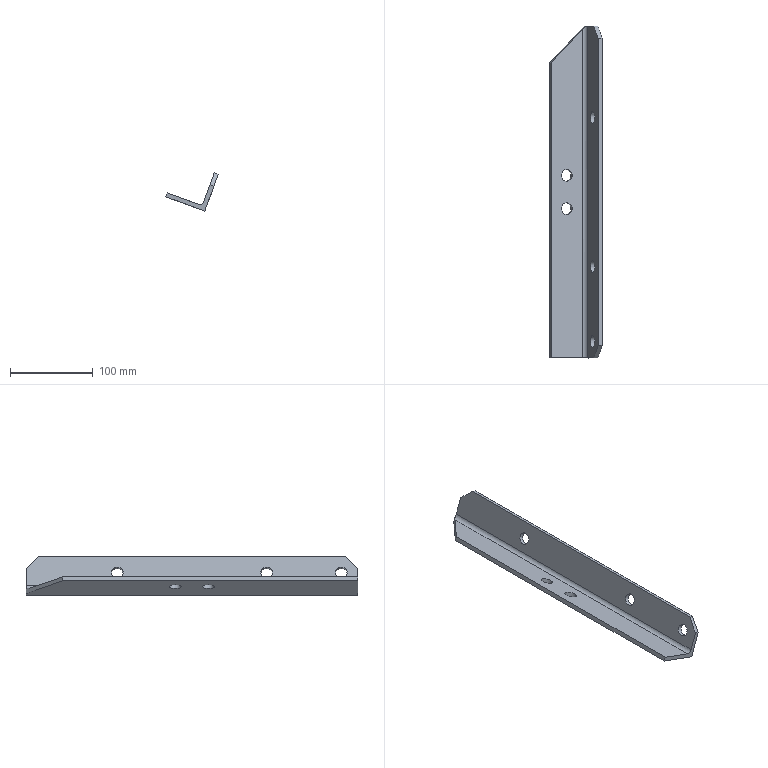Part | NX | features solid 2 | 1 solid | 17 faces | box 63.06 x 400 x 45.876 mm | volume 176299 mm3 | plane 11 | cylinder 6 | commonest cylinder face diameters 14 x5 10 x1
STEP:
#1=CARTESIAN_POINT('',(-698.232,-745.,85.667));
#2=VERTEX_POINT('',#1);
#3=CARTESIAN_POINT('',(-695.838,-745.,92.245));
#4=DIRECTION('',(0.9397,0.,-0.342));
#5=DIRECTION('',(-0.342,0.,-0.9397));
#6=AXIS2_PLACEMENT_3D('',#3,#4,#5);
#7=CIRCLE('',#6,7.);
#8=EDGE_CURVE('',#2,#2,#7,.F.);
#9=ORIENTED_EDGE('',*,*,#8,.F.);
#10=EDGE_LOOP('',(#9));
#11=FACE_BOUND('',#10,.T.);
#12=CARTESIAN_POINT('',(-698.232,-925.,85.667));
#13=VERTEX_POINT('',#12);
#14=CARTESIAN_POINT('',(-695.838,-925.,92.245));
#15=DIRECTION('',(0.9397,0.,-0.342));
#16=DIRECTION('',(-0.342,0.,-0.9397));
#17=AXIS2_PLACEMENT_3D('',#14,#15,#16);
#18=CIRCLE('',#17,7.);
#19=EDGE_CURVE('',#13,#13,#18,.F.);
#20=ORIENTED_EDGE('',*,*,#19,.F.);
#21=EDGE_LOOP('',(#20));
#22=FACE_BOUND('',#21,.T.);
#23=CARTESIAN_POINT('',(-694.127,-1035.,96.944));
#24=VERTEX_POINT('',#23);
#25=CARTESIAN_POINT('',(-701.652,-1035.,76.27));
#26=VERTEX_POINT('',#25);
#27=CARTESIAN_POINT('',(-693.101,-1035.,99.763));
#28=DIRECTION('',(-0.342,0.,-0.9397));
#29=VECTOR('',#28,1000.);
#30=LINE('',#27,#29);
#31=EDGE_CURVE('',#24,#26,#30,.T.);
#32=ORIENTED_EDGE('',*,*,#31,.F.);
#33=CARTESIAN_POINT('',(-688.997,-1020.,111.039));
#34=VERTEX_POINT('',#33);
#35=CARTESIAN_POINT('',(-663.625,-945.818,180.748));
#36=DIRECTION('',(0.2418,0.7071,0.6645));
#37=VECTOR('',#36,1000.);
#38=LINE('',#35,#37);
#39=EDGE_CURVE('',#24,#34,#38,.T.);
#40=ORIENTED_EDGE('',*,*,#39,.T.);
#41=CARTESIAN_POINT('',(-688.997,-650.,111.039));
#42=VERTEX_POINT('',#41);
#43=CARTESIAN_POINT('',(-688.997,-859.636,111.039));
#44=DIRECTION('',(0.,-1.,0.));
#45=VECTOR('',#44,1000.);
#46=LINE('',#43,#45);
#47=EDGE_CURVE('',#42,#34,#46,.T.);
#48=ORIENTED_EDGE('',*,*,#47,.F.);
#49=CARTESIAN_POINT('',(-694.127,-635.,96.944));
#50=VERTEX_POINT('',#49);
#51=CARTESIAN_POINT('',(-670.59,-703.818,161.611));
#52=DIRECTION('',(0.2418,-0.7071,0.6645));
#53=VECTOR('',#52,1000.);
#54=LINE('',#51,#53);
#55=EDGE_CURVE('',#42,#50,#54,.F.);
#56=ORIENTED_EDGE('',*,*,#55,.T.);
#57=CARTESIAN_POINT('',(-701.652,-635.,76.27));
#58=VERTEX_POINT('',#57);
#59=CARTESIAN_POINT('',(-695.838,-635.,92.245));
#60=DIRECTION('',(0.342,0.,0.9397));
#61=VECTOR('',#60,1000.);
#62=LINE('',#59,#61);
#63=EDGE_CURVE('',#58,#50,#62,.T.);
#64=ORIENTED_EDGE('',*,*,#63,.F.);
#65=CARTESIAN_POINT('',(-701.652,-1074.813,76.27));
#66=DIRECTION('',(0.,-1.,0.));
#67=VECTOR('',#66,1000.);
#68=LINE('',#65,#67);
#69=EDGE_CURVE('',#58,#26,#68,.T.);
#70=ORIENTED_EDGE('',*,*,#69,.T.);
#71=EDGE_LOOP('',(#32,#40,#48,#56,#64,#70));
#72=FACE_BOUND('',#71,.T.);
#73=CARTESIAN_POINT('',(-693.443,-1015.,98.823));
#74=VERTEX_POINT('',#73);
#75=CARTESIAN_POINT('',(-695.838,-1015.,92.245));
#76=DIRECTION('',(-0.9397,0.,0.342));
#77=DIRECTION('',(0.342,0.,0.9397));
#78=AXIS2_PLACEMENT_3D('',#75,#76,#77);
#79=CIRCLE('',#78,7.);
#80=EDGE_CURVE('',#74,#74,#79,.F.);
#81=ORIENTED_EDGE('',*,*,#80,.T.);
#82=EDGE_LOOP('',(#81));
#83=FACE_BOUND('',#82,.T.);
#84=CARTESIAN_POINT('',(-693.101,-859.636,99.763));
#85=DIRECTION('',(-0.9397,0.,0.342));
#86=DIRECTION('',(-0.342,0.,-0.9397));
#87=AXIS2_PLACEMENT_3D('',#84,#85,#86);
#88=PLANE('',#87);
#89=ADVANCED_FACE('',(#11,#22,#72,#83),#88,.T.);
#90=CARTESIAN_POINT('',(-688.745,-745.,97.113));
#91=VERTEX_POINT('',#90);
#92=CARTESIAN_POINT('',(-691.139,-745.,90.535));
#93=DIRECTION('',(-0.9397,0.,0.342));
#94=DIRECTION('',(0.342,0.,0.9397));
#95=AXIS2_PLACEMENT_3D('',#92,#93,#94);
#96=CIRCLE('',#95,7.);
#97=EDGE_CURVE('',#91,#91,#96,.F.);
#98=ORIENTED_EDGE('',*,*,#97,.F.);
#99=EDGE_LOOP('',(#98));
#100=FACE_BOUND('',#99,.T.);
#101=CARTESIAN_POINT('',(-688.745,-925.,97.113));
#102=VERTEX_POINT('',#101);
#103=CARTESIAN_POINT('',(-691.139,-925.,90.535));
#104=DIRECTION('',(-0.9397,0.,0.342));
#105=DIRECTION('',(0.342,0.,0.9397));
#106=AXIS2_PLACEMENT_3D('',#103,#104,#105);
#107=CIRCLE('',#106,7.);
#108=EDGE_CURVE('',#102,#102,#107,.F.);
#109=ORIENTED_EDGE('',*,*,#108,.F.);
#110=EDGE_LOOP('',(#109));
#111=FACE_BOUND('',#110,.T.);
#112=CARTESIAN_POINT('',(-684.299,-650.,109.329));
#113=VERTEX_POINT('',#112);
#114=CARTESIAN_POINT('',(-684.299,-1020.,109.329));
#115=VERTEX_POINT('',#114);
#116=CARTESIAN_POINT('',(-684.299,-859.636,109.329));
#117=DIRECTION('',(0.,-1.,0.));
#118=VECTOR('',#117,1000.);
#119=LINE('',#116,#118);
#120=EDGE_CURVE('',#113,#115,#119,.T.);
#121=ORIENTED_EDGE('',*,*,#120,.T.);
#122=CARTESIAN_POINT('',(-689.429,-1035.,95.234));
#123=VERTEX_POINT('',#122);
#124=CARTESIAN_POINT('',(-658.927,-945.818,179.037));
#125=DIRECTION('',(-0.2418,-0.7071,-0.6645));
#126=VECTOR('',#125,1000.);
#127=LINE('',#124,#126);
#128=EDGE_CURVE('',#115,#123,#127,.T.);
#129=ORIENTED_EDGE('',*,*,#128,.T.);
#130=CARTESIAN_POINT('',(-700.374,-1035.,65.163));
#131=VERTEX_POINT('',#130);
#132=CARTESIAN_POINT('',(-688.403,-1035.,98.053));
#133=DIRECTION('',(0.342,0.,0.9397));
#134=VECTOR('',#133,1000.);
#135=LINE('',#132,#134);
#136=EDGE_CURVE('',#131,#123,#135,.T.);
#137=ORIENTED_EDGE('',*,*,#136,.F.);
#138=CARTESIAN_POINT('',(-700.374,-635.,65.163));
#139=VERTEX_POINT('',#138);
#140=CARTESIAN_POINT('',(-700.374,-859.636,65.163));
#141=DIRECTION('',(0.,-1.,0.));
#142=VECTOR('',#141,1000.);
#143=LINE('',#140,#142);
#144=EDGE_CURVE('',#139,#131,#143,.T.);
#145=ORIENTED_EDGE('',*,*,#144,.F.);
#146=CARTESIAN_POINT('',(-689.429,-635.,95.234));
#147=VERTEX_POINT('',#146);
#148=CARTESIAN_POINT('',(-691.139,-635.,90.535));
#149=DIRECTION('',(-0.342,0.,-0.9397));
#150=VECTOR('',#149,1000.);
#151=LINE('',#148,#150);
#152=EDGE_CURVE('',#147,#139,#151,.T.);
#153=ORIENTED_EDGE('',*,*,#152,.F.);
#154=CARTESIAN_POINT('',(-665.892,-703.818,159.901));
#155=DIRECTION('',(-0.2418,0.7071,-0.6645));
#156=VECTOR('',#155,1000.);
#157=LINE('',#154,#156);
#158=EDGE_CURVE('',#147,#113,#157,.F.);
#159=ORIENTED_EDGE('',*,*,#158,.T.);
#160=EDGE_LOOP('',(#121,#129,#137,#145,#153,#159));
#161=FACE_BOUND('',#160,.T.);
#162=CARTESIAN_POINT('',(-693.533,-1015.,83.957));
#163=VERTEX_POINT('',#162);
#164=CARTESIAN_POINT('',(-691.139,-1015.,90.535));
#165=DIRECTION('',(0.9397,0.,-0.342));
#166=DIRECTION('',(-0.342,0.,-0.9397));
#167=AXIS2_PLACEMENT_3D('',#164,#165,#166);
#168=CIRCLE('',#167,7.);
#169=EDGE_CURVE('',#163,#163,#168,.T.);
#170=ORIENTED_EDGE('',*,*,#169,.F.);
#171=EDGE_LOOP('',(#170));
#172=FACE_BOUND('',#171,.T.);
#173=CARTESIAN_POINT('',(-688.403,-859.636,98.053));
#174=DIRECTION('',(0.9397,0.,-0.342));
#175=DIRECTION('',(0.342,0.,0.9397));
#176=AXIS2_PLACEMENT_3D('',#173,#174,#175);
#177=PLANE('',#176);
#178=ADVANCED_FACE('',(#100,#111,#161,#172),#177,.T.);
#179=ORIENTED_EDGE('',*,*,#47,.T.);
#180=CARTESIAN_POINT('',(-684.299,-1020.,109.329));
#181=DIRECTION('',(0.9397,0.,-0.342));
#182=VECTOR('',#181,1000.);
#183=LINE('',#180,#182);
#184=EDGE_CURVE('',#34,#115,#183,.T.);
#185=ORIENTED_EDGE('',*,*,#184,.T.);
#186=ORIENTED_EDGE('',*,*,#120,.F.);
#187=CARTESIAN_POINT('',(-693.696,-650.,112.749));
#188=DIRECTION('',(-0.9397,0.,0.342));
#189=VECTOR('',#188,1000.);
#190=LINE('',#187,#189);
#191=EDGE_CURVE('',#113,#42,#190,.T.);
#192=ORIENTED_EDGE('',*,*,#191,.T.);
#193=EDGE_LOOP('',(#179,#185,#186,#192));
#194=FACE_BOUND('',#193,.T.);
#195=CARTESIAN_POINT('',(-693.696,-859.636,112.749));
#196=DIRECTION('',(0.342,0.,0.9397));
#197=DIRECTION('',(0.,-1.,0.));
#198=AXIS2_PLACEMENT_3D('',#195,#196,#197);
#199=PLANE('',#198);
#200=ADVANCED_FACE('',(#194),#199,.T.);
#201=CARTESIAN_POINT('',(-708.06,-1035.,73.282));
#202=VERTEX_POINT('',#201);
#203=CARTESIAN_POINT('',(-708.06,-639.142,73.282));
#204=VERTEX_POINT('',#203);
#205=CARTESIAN_POINT('',(-708.06,-740.,73.282));
#206=DIRECTION('',(0.,-1.,0.));
#207=VECTOR('',#206,1000.);
#208=LINE('',#205,#207);
#209=EDGE_CURVE('',#202,#204,#208,.F.);
#210=ORIENTED_EDGE('',*,*,#209,.F.);
#211=CARTESIAN_POINT('',(-706.35,-1035.,77.981));
#212=DIRECTION('',(0.,1.,0.));
#213=DIRECTION('',(-0.08716,0.,0.9962));
#214=AXIS2_PLACEMENT_3D('',#211,#212,#213);
#215=CIRCLE('',#214,5.);
#216=EDGE_CURVE('',#202,#26,#215,.F.);
#217=ORIENTED_EDGE('',*,*,#216,.T.);
#218=ORIENTED_EDGE('',*,*,#69,.F.);
#219=CARTESIAN_POINT('',(-703.416,-635.,73.932));
#220=VERTEX_POINT('',#219);
#221=CARTESIAN_POINT('',(-706.35,-635.,77.981));
#222=DIRECTION('',(0.,1.,0.));
#223=DIRECTION('',(-0.9962,0.,-0.08716));
#224=AXIS2_PLACEMENT_3D('',#221,#222,#223);
#225=CIRCLE('',#224,5.);
#226=EDGE_CURVE('',#58,#220,#225,.T.);
#227=ORIENTED_EDGE('',*,*,#226,.T.);
#228=CARTESIAN_POINT('',(-706.35,-639.142,77.981));
#229=DIRECTION('',(0.6645,-0.7071,-0.2418));
#230=DIRECTION('',(0.6645,0.7071,-0.2418));
#231=AXIS2_PLACEMENT_3D('',#228,#229,#230);
#232=ELLIPSE('',#231,7.071,5.);
#233=EDGE_CURVE('',#204,#220,#232,.T.);
#234=ORIENTED_EDGE('',*,*,#233,.F.);
#235=EDGE_LOOP('',(#210,#217,#218,#227,#234));
#236=FACE_BOUND('',#235,.T.);
#237=CARTESIAN_POINT('',(-706.35,-859.636,77.981));
#238=DIRECTION('',(0.,1.,0.));
#239=DIRECTION('',(-0.342,0.,-0.9397));
#240=AXIS2_PLACEMENT_3D('',#237,#238,#239);
#241=CYLINDRICAL_SURFACE('',#240,5.);
#242=ADVANCED_FACE('',(#236),#241,.F.);
#243=CARTESIAN_POINT('',(-745.648,-679.142,86.963));
#244=VERTEX_POINT('',#243);
#245=CARTESIAN_POINT('',(-745.648,-1035.,86.963));
#246=VERTEX_POINT('',#245);
#247=CARTESIAN_POINT('',(-745.648,-859.636,86.963));
#248=DIRECTION('',(0.,-1.,0.));
#249=VECTOR('',#248,1000.);
#250=LINE('',#247,#249);
#251=EDGE_CURVE('',#244,#246,#250,.T.);
#252=ORIENTED_EDGE('',*,*,#251,.F.);
#253=CARTESIAN_POINT('',(-747.358,-679.142,82.264));
#254=VERTEX_POINT('',#253);
#255=CARTESIAN_POINT('',(-735.388,-679.142,115.154));
#256=DIRECTION('',(0.342,0.,0.9397));
#257=VECTOR('',#256,1000.);
#258=LINE('',#255,#257);
#259=EDGE_CURVE('',#244,#254,#258,.F.);
#260=ORIENTED_EDGE('',*,*,#259,.T.);
#261=CARTESIAN_POINT('',(-747.358,-1035.,82.264));
#262=VERTEX_POINT('',#261);
#263=CARTESIAN_POINT('',(-747.358,-857.5,82.264));
#264=DIRECTION('',(0.,-1.,0.));
#265=VECTOR('',#264,1000.);
#266=LINE('',#263,#265);
#267=EDGE_CURVE('',#254,#262,#266,.T.);
#268=ORIENTED_EDGE('',*,*,#267,.T.);
#269=CARTESIAN_POINT('',(-735.388,-1035.,115.154));
#270=DIRECTION('',(-0.342,0.,-0.9397));
#271=VECTOR('',#270,1000.);
#272=LINE('',#269,#271);
#273=EDGE_CURVE('',#246,#262,#272,.T.);
#274=ORIENTED_EDGE('',*,*,#273,.F.);
#275=EDGE_LOOP('',(#252,#260,#268,#274));
#276=FACE_BOUND('',#275,.T.);
#277=CARTESIAN_POINT('',(-735.388,-859.636,115.154));
#278=DIRECTION('',(-0.9397,0.,0.342));
#279=DIRECTION('',(-0.342,0.,-0.9397));
#280=AXIS2_PLACEMENT_3D('',#277,#278,#279);
#281=PLANE('',#280);
#282=ADVANCED_FACE('',(#276),#281,.T.);
#283=CARTESIAN_POINT('',(-733.432,-815.,82.517));
#284=VERTEX_POINT('',#283);
#285=CARTESIAN_POINT('',(-726.854,-815.,80.122));
#286=DIRECTION('',(-0.342,0.,-0.9397));
#287=DIRECTION('',(-0.9397,0.,0.342));
#288=AXIS2_PLACEMENT_3D('',#285,#286,#287);
#289=CIRCLE('',#288,7.);
#290=EDGE_CURVE('',#284,#284,#289,.T.);
#291=ORIENTED_EDGE('',*,*,#290,.T.);
#292=EDGE_LOOP('',(#291));
#293=FACE_BOUND('',#292,.T.);
#294=CARTESIAN_POINT('',(-733.432,-855.,82.517));
#295=VERTEX_POINT('',#294);
#296=CARTESIAN_POINT('',(-726.854,-855.,80.122));
#297=DIRECTION('',(-0.342,0.,-0.9397));
#298=DIRECTION('',(-0.9397,0.,0.342));
#299=AXIS2_PLACEMENT_3D('',#296,#297,#298);
#300=CIRCLE('',#299,7.);
#301=EDGE_CURVE('',#295,#295,#300,.T.);
#302=ORIENTED_EDGE('',*,*,#301,.T.);
#303=EDGE_LOOP('',(#302));
#304=FACE_BOUND('',#303,.T.);
#305=ORIENTED_EDGE('',*,*,#209,.T.);
#306=CARTESIAN_POINT('',(-829.592,-768.474,117.516));
#307=DIRECTION('',(0.6645,0.7071,-0.2418));
#308=VECTOR('',#307,1000.);
#309=LINE('',#306,#308);
#310=EDGE_CURVE('',#204,#244,#309,.F.);
#311=ORIENTED_EDGE('',*,*,#310,.T.);
#312=ORIENTED_EDGE('',*,*,#251,.T.);
#313=CARTESIAN_POINT('',(-745.648,-1035.,86.963));
#314=DIRECTION('',(-0.9397,0.,0.342));
#315=VECTOR('',#314,1000.);
#316=LINE('',#313,#315);
#317=EDGE_CURVE('',#202,#246,#316,.T.);
#318=ORIENTED_EDGE('',*,*,#317,.F.);
#319=EDGE_LOOP('',(#305,#311,#312,#318));
#320=FACE_BOUND('',#319,.T.);
#321=CARTESIAN_POINT('',(-745.648,-857.805,86.963));
#322=DIRECTION('',(0.342,0.,0.9397));
#323=DIRECTION('',(0.,-1.,0.));
#324=AXIS2_PLACEMENT_3D('',#321,#322,#323);
#325=PLANE('',#324);
#326=ADVANCED_FACE('',(#293,#304,#320),#325,.T.);
#327=CARTESIAN_POINT('',(-735.142,-815.,77.818));
#328=VERTEX_POINT('',#327);
#329=CARTESIAN_POINT('',(-728.564,-815.,75.424));
#330=DIRECTION('',(-0.342,0.,-0.9397));
#331=DIRECTION('',(-0.9397,0.,0.342));
#332=AXIS2_PLACEMENT_3D('',#329,#330,#331);
#333=CIRCLE('',#332,7.);
#334=EDGE_CURVE('',#328,#328,#333,.T.);
#335=ORIENTED_EDGE('',*,*,#334,.F.);
#336=EDGE_LOOP('',(#335));
#337=FACE_BOUND('',#336,.T.);
#338=CARTESIAN_POINT('',(-735.142,-855.,77.818));
#339=VERTEX_POINT('',#338);
#340=CARTESIAN_POINT('',(-728.564,-855.,75.424));
#341=DIRECTION('',(-0.342,0.,-0.9397));
#342=DIRECTION('',(-0.9397,0.,0.342));
#343=AXIS2_PLACEMENT_3D('',#340,#341,#342);
#344=CIRCLE('',#343,7.);
#345=EDGE_CURVE('',#339,#339,#344,.T.);
#346=ORIENTED_EDGE('',*,*,#345,.F.);
#347=EDGE_LOOP('',(#346));
#348=FACE_BOUND('',#347,.T.);
#349=ORIENTED_EDGE('',*,*,#267,.F.);
#350=CARTESIAN_POINT('',(-705.878,-635.,67.167));
#351=VERTEX_POINT('',#350);
#352=CARTESIAN_POINT('',(-810.016,-745.821,105.07));
#353=DIRECTION('',(-0.6645,-0.7071,0.2418));
#354=VECTOR('',#353,1000.);
#355=LINE('',#352,#354);
#356=EDGE_CURVE('',#254,#351,#355,.F.);
#357=ORIENTED_EDGE('',*,*,#356,.T.);
#358=CARTESIAN_POINT('',(-705.072,-635.,66.874));
#359=DIRECTION('',(-0.9397,0.,0.342));
#360=VECTOR('',#359,1000.);
#361=LINE('',#358,#360);
#362=EDGE_CURVE('',#139,#351,#361,.T.);
#363=ORIENTED_EDGE('',*,*,#362,.F.);
#364=ORIENTED_EDGE('',*,*,#144,.T.);
#365=CARTESIAN_POINT('',(-705.072,-1035.,66.874));
#366=DIRECTION('',(0.9397,0.,-0.342));
#367=VECTOR('',#366,1000.);
#368=LINE('',#365,#367);
#369=EDGE_CURVE('',#262,#131,#368,.T.);
#370=ORIENTED_EDGE('',*,*,#369,.F.);
#371=EDGE_LOOP('',(#349,#357,#363,#364,#370));
#372=FACE_BOUND('',#371,.T.);
#373=CARTESIAN_POINT('',(-705.072,-857.5,66.874));
#374=DIRECTION('',(-0.342,0.,-0.9397));
#375=DIRECTION('',(0.,1.,0.));
#376=AXIS2_PLACEMENT_3D('',#373,#374,#375);
#377=PLANE('',#376);
#378=ADVANCED_FACE('',(#337,#348,#372),#377,.T.);
#379=ORIENTED_EDGE('',*,*,#19,.T.);
#380=EDGE_LOOP('',(#379));
#381=FACE_BOUND('',#380,.T.);
#382=ORIENTED_EDGE('',*,*,#108,.T.);
#383=EDGE_LOOP('',(#382));
#384=FACE_BOUND('',#383,.T.);
#385=CARTESIAN_POINT('',(-719.33,-925.,100.796));
#386=DIRECTION('',(0.9397,0.,-0.342));
#387=DIRECTION('',(0.,-1.,0.));
#388=AXIS2_PLACEMENT_3D('',#385,#386,#387);
#389=CYLINDRICAL_SURFACE('',#388,7.);
#390=ADVANCED_FACE('',(#381,#384),#389,.F.);
#391=ORIENTED_EDGE('',*,*,#136,.T.);
#392=CARTESIAN_POINT('',(-694.127,-1035.,96.944));
#393=DIRECTION('',(-0.9397,0.,0.342));
#394=VECTOR('',#393,1000.);
#395=LINE('',#392,#394);
#396=EDGE_CURVE('',#123,#24,#395,.T.);
#397=ORIENTED_EDGE('',*,*,#396,.T.);
#398=ORIENTED_EDGE('',*,*,#31,.T.);
#399=ORIENTED_EDGE('',*,*,#216,.F.);
#400=ORIENTED_EDGE('',*,*,#317,.T.);
#401=ORIENTED_EDGE('',*,*,#273,.T.);
#402=ORIENTED_EDGE('',*,*,#369,.T.);
#403=EDGE_LOOP('',(#391,#397,#398,#399,#400,#401,#402));
#404=FACE_BOUND('',#403,.T.);
#405=CARTESIAN_POINT('',(-118.087,-1035.,-25.569));
#406=DIRECTION('',(0.,1.,0.));
#407=DIRECTION('',(-0.08716,0.,0.9962));
#408=AXIS2_PLACEMENT_3D('',#405,#406,#407);
#409=PLANE('',#408);
#410=ADVANCED_FACE('',(#404),#409,.F.);
#411=ORIENTED_EDGE('',*,*,#362,.T.);
#412=CARTESIAN_POINT('',(-696.644,-635.,92.539));
#413=DIRECTION('',(-0.342,0.,-0.9397));
#414=VECTOR('',#413,1000.);
#415=LINE('',#412,#414);
#416=EDGE_CURVE('',#351,#220,#415,.F.);
#417=ORIENTED_EDGE('',*,*,#416,.T.);
#418=ORIENTED_EDGE('',*,*,#226,.F.);
#419=ORIENTED_EDGE('',*,*,#63,.T.);
#420=CARTESIAN_POINT('',(-694.127,-635.,96.944));
#421=DIRECTION('',(0.9397,0.,-0.342));
#422=VECTOR('',#421,1000.);
#423=LINE('',#420,#422);
#424=EDGE_CURVE('',#50,#147,#423,.T.);
#425=ORIENTED_EDGE('',*,*,#424,.T.);
#426=ORIENTED_EDGE('',*,*,#152,.T.);
#427=EDGE_LOOP('',(#411,#417,#418,#419,#425,#426));
#428=FACE_BOUND('',#427,.T.);
#429=CARTESIAN_POINT('',(-695.838,-635.,92.245));
#430=DIRECTION('',(0.,1.,0.));
#431=DIRECTION('',(0.7071,0.,-0.7071));
#432=AXIS2_PLACEMENT_3D('',#429,#430,#431);
#433=PLANE('',#432);
#434=ADVANCED_FACE('',(#428),#433,.T.);
#435=ORIENTED_EDGE('',*,*,#8,.T.);
#436=EDGE_LOOP('',(#435));
#437=FACE_BOUND('',#436,.T.);
#438=ORIENTED_EDGE('',*,*,#97,.T.);
#439=EDGE_LOOP('',(#438));
#440=FACE_BOUND('',#439,.T.);
#441=CARTESIAN_POINT('',(-719.33,-745.,100.796));
#442=DIRECTION('',(0.9397,0.,-0.342));
#443=DIRECTION('',(0.,-1.,0.));
#444=AXIS2_PLACEMENT_3D('',#441,#442,#443);
#445=CYLINDRICAL_SURFACE('',#444,7.);
#446=ADVANCED_FACE('',(#437,#440),#445,.F.);
#447=ORIENTED_EDGE('',*,*,#80,.F.);
#448=EDGE_LOOP('',(#447));
#449=FACE_BOUND('',#448,.T.);
#450=ORIENTED_EDGE('',*,*,#169,.T.);
#451=EDGE_LOOP('',(#450));
#452=FACE_BOUND('',#451,.T.);
#453=CARTESIAN_POINT('',(-719.33,-1015.,100.796));
#454=DIRECTION('',(0.9397,0.,-0.342));
#455=DIRECTION('',(0.,-1.,0.));
#456=AXIS2_PLACEMENT_3D('',#453,#454,#455);
#457=CYLINDRICAL_SURFACE('',#456,7.);
#458=ADVANCED_FACE('',(#449,#452),#457,.F.);
#459=ORIENTED_EDGE('',*,*,#128,.F.);
#460=ORIENTED_EDGE('',*,*,#184,.F.);
#461=ORIENTED_EDGE('',*,*,#39,.F.);
#462=ORIENTED_EDGE('',*,*,#396,.F.);
#463=EDGE_LOOP('',(#459,#460,#461,#462));
#464=FACE_BOUND('',#463,.T.);
#465=CARTESIAN_POINT('',(-146.096,-1035.,-102.524));
#466=DIRECTION('',(0.2418,-0.7071,0.6645));
#467=DIRECTION('',(0.06458,-0.6715,-0.7381));
#468=AXIS2_PLACEMENT_3D('',#465,#466,#467);
#469=PLANE('',#468);
#470=ADVANCED_FACE('',(#464),#469,.T.);
#471=ORIENTED_EDGE('',*,*,#55,.F.);
#472=ORIENTED_EDGE('',*,*,#191,.F.);
#473=ORIENTED_EDGE('',*,*,#158,.F.);
#474=ORIENTED_EDGE('',*,*,#424,.F.);
#475=EDGE_LOOP('',(#471,#472,#473,#474));
#476=FACE_BOUND('',#475,.T.);
#477=CARTESIAN_POINT('',(-694.127,-635.,96.944));
#478=DIRECTION('',(-0.2418,-0.7071,-0.6645));
#479=DIRECTION('',(0.06458,0.6715,-0.7381));
#480=AXIS2_PLACEMENT_3D('',#477,#478,#479);
#481=PLANE('',#480);
#482=ADVANCED_FACE('',(#476),#481,.F.);
#483=ORIENTED_EDGE('',*,*,#345,.T.);
#484=EDGE_LOOP('',(#483));
#485=FACE_BOUND('',#484,.T.);
#486=ORIENTED_EDGE('',*,*,#301,.F.);
#487=EDGE_LOOP('',(#486));
#488=FACE_BOUND('',#487,.T.);
#489=CARTESIAN_POINT('',(-726.854,-855.,80.122));
#490=DIRECTION('',(-0.342,0.,-0.9397));
#491=DIRECTION('',(-0.9397,0.,0.342));
#492=AXIS2_PLACEMENT_3D('',#489,#490,#491);
#493=CYLINDRICAL_SURFACE('',#492,7.);
#494=ADVANCED_FACE('',(#485,#488),#493,.F.);
#495=ORIENTED_EDGE('',*,*,#334,.T.);
#496=EDGE_LOOP('',(#495));
#497=FACE_BOUND('',#496,.T.);
#498=ORIENTED_EDGE('',*,*,#290,.F.);
#499=EDGE_LOOP('',(#498));
#500=FACE_BOUND('',#499,.T.);
#501=CARTESIAN_POINT('',(-726.854,-815.,80.122));
#502=DIRECTION('',(-0.342,0.,-0.9397));
#503=DIRECTION('',(-0.9397,0.,0.342));
#504=AXIS2_PLACEMENT_3D('',#501,#502,#503);
#505=CYLINDRICAL_SURFACE('',#504,7.);
#506=ADVANCED_FACE('',(#497,#500),#505,.F.);
#507=ORIENTED_EDGE('',*,*,#356,.F.);
#508=ORIENTED_EDGE('',*,*,#259,.F.);
#509=ORIENTED_EDGE('',*,*,#310,.F.);
#510=ORIENTED_EDGE('',*,*,#233,.T.);
#511=ORIENTED_EDGE('',*,*,#416,.F.);
#512=EDGE_LOOP('',(#507,#508,#509,#510,#511));
#513=FACE_BOUND('',#512,.T.);
#514=CARTESIAN_POINT('',(-703.288,-642.071,94.957));
#515=DIRECTION('',(0.6645,-0.7071,-0.2418));
#516=DIRECTION('',(0.7287,0.6848,0.));
#517=AXIS2_PLACEMENT_3D('',#514,#515,#516);
#518=PLANE('',#517);
#519=ADVANCED_FACE('',(#513),#518,.F.);
#520=CLOSED_SHELL('',(#89,#178,#200,#242,#282,#326,#378,#390,#410,#434,#446,#458,#470,#482,#494,#506,#519));
#521=MANIFOLD_SOLID_BREP('',#520);
#522=(LENGTH_UNIT()NAMED_UNIT(*)SI_UNIT(.MILLI.,.METRE.));
#523=UNCERTAINTY_MEASURE_WITH_UNIT(LENGTH_MEASURE(0.00001),#522,'','');
#524=(NAMED_UNIT(*)PLANE_ANGLE_UNIT()SI_UNIT($,.RADIAN.));
#525=(NAMED_UNIT(*)SI_UNIT($,.STERADIAN.)SOLID_ANGLE_UNIT());
#526=(GEOMETRIC_REPRESENTATION_CONTEXT(3)GLOBAL_UNCERTAINTY_ASSIGNED_CONTEXT((#523))GLOBAL_UNIT_ASSIGNED_CONTEXT((#522,#524,#525))REPRESENTATION_CONTEXT('',''));
#527=ADVANCED_BREP_SHAPE_REPRESENTATION('',(#521),#526);